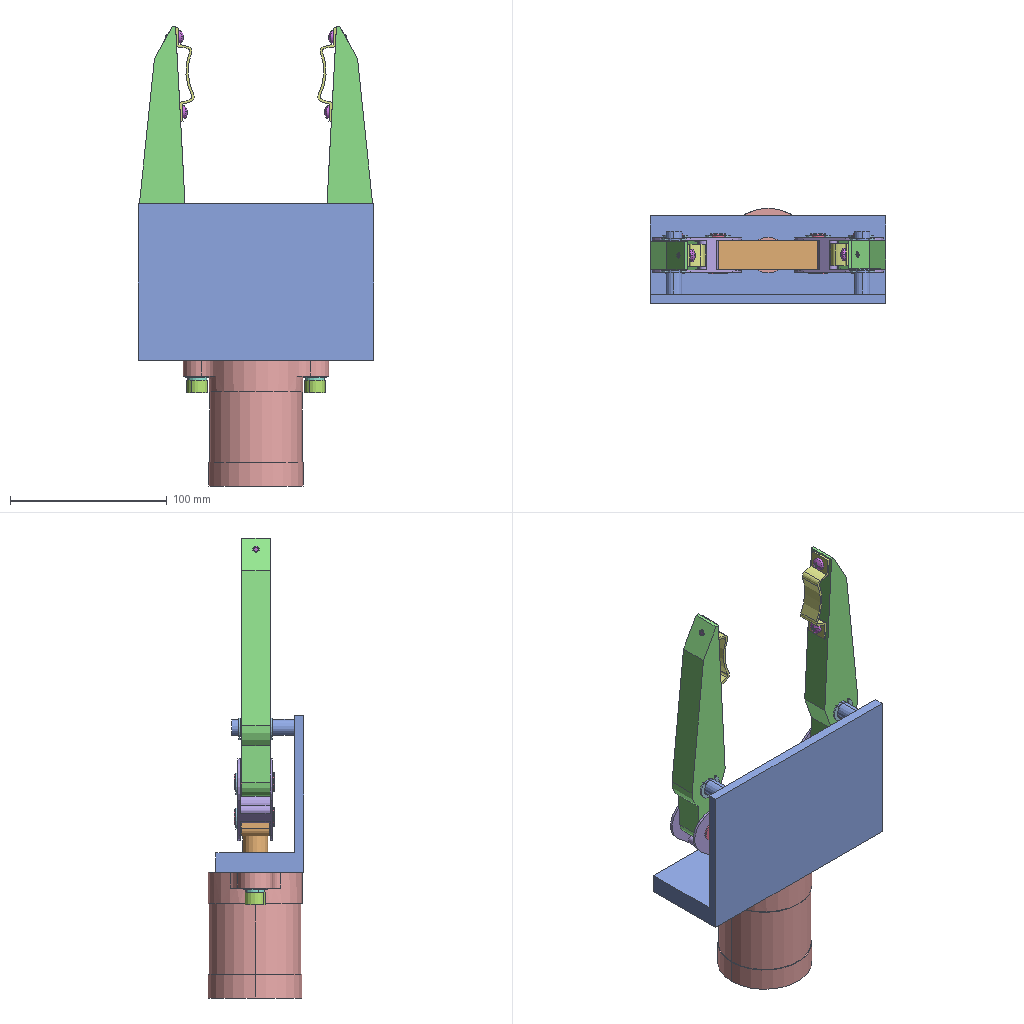Assembly | SolidWorks | 12 different items | 31 placed | box 150 x 61 x 293 mm
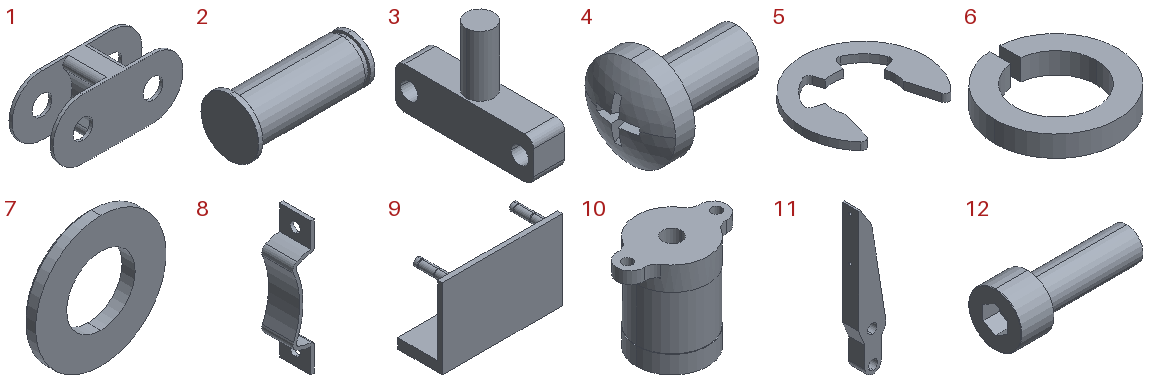Parts list (item | quantity | size | volume | features):
1 | x2 | 65 x 22 x 30 mm | 10120 mm3 | features Extrusion 1, Fillet 1, ICE 1
2 | x4 | 25.5 x 12 x 12 mm | 1834 mm3 | features Chamfer 2, ICE 2, Extrusion 1, Fillet 1
3 | x1 | 18 x 80 x 59 mm | 38383 mm3 | features ICE 2, Extrusion 1, Fillet 1
4 | x4 | 11.081 x 8 x 8 mm | 215 mm3 | features BlendCut 1, LPattern 1, MirrorPattern 1, RevCut 1, Revolution 1
5 | x8 | 16 x 13.638 x 1 mm | 90.427 mm3 | features Extrusion 1
6 | x2 | 12.277 x 12.254 x 2.1 mm | 135.755 mm3 | features Extrusion 1
7 | x2 | 16 x 1.6 x 16 mm | 229.077 mm3 | features Revolution 1
8 | x2 | 9.547 x 14 x 60 mm | 1466 mm3 | features ExtruThin 1, ICE 1
9 | x1 | 150 x 56 x 100 mm | 183819 mm3 | features Cut 3, ICE 2, 3DProfileFeature 1, Extrusion 1, HoleWzd 1
10 | x1 | 92.5 x 60 x 80 mm | 214232 mm3 | features ICE 5, Cut 2, Extrusion 1, Fillet 1
11 | x2 | 30.153 x 18 x 164 mm | 54880 mm3 | features 3DProfileFeature 1, Extrusion 1, HoleWzd 1
12 | x2 | 33 x 13 x 13 mm | 2189 mm3 | features BlendCut 1, Cut 1, Fillet 1, LPattern 1, RevCut 1, Revolution 1
Mates (type | each side: item.copy, entity, surface, feature):
Concentric | 10.1 face cylinder Cut-Extrude1 | 9.1 face cylinder Boss-Extrude1
Coincident | 10.1 face plane Boss-Extrude1 | 9.1 face plane Boss-Extrude1
Concentric | 10.1 face cylinder Cut-Extrude2 | 12.1 face cylinder Base-Revolve
Coincident | 10.1 face plane Cut-Extrude3 | 7.1 face plane Base-Revolve | 2 times
Coincident | 7.1 face plane Base-Revolve | 6.1 face plane Extrude1
Concentric | 7.1 face cylinder Base-Revolve | 6.1 face cylinder Extrude1
Concentric | 10.1 face cylinder Cut-Extrude2 | 6.1 face cylinder Extrude1
Coincident | 12.1 face plane Base-Revolve | 6.1 face plane Extrude1
Concentric | 10.1 face cylinder Cut-Extrude1 | 3.1 face cylinder Boss-Extrude1
Parallel | 9.1 face plane Boss-Extrude2 | 3.1 face plane Boss-Extrude2
Concentric | 3.1 face cylinder Cut-Extrude1 | 1.1 face cylinder Boss-Extrude2
DistanceDim | 1.1 face plane Cut-Extrude1 | 3.1 face plane Boss-Extrude2
DistanceDim | 1.2 face plane Cut-Extrude1 | 3.1 face plane Boss-Extrude2
Concentric | 3.1 face cylinder Cut-Extrude1 | 1.2 face cylinder Boss-Extrude2
Concentric | 1.2 face cylinder Boss-Extrude2 | 11.1 face cylinder Boss-Extrude1
DistanceDim | 11.1 face plane Boss-Extrude1 | 1.2 face plane Cut-Extrude1
Concentric | 10.1 face cylinder Cut-Extrude2 | 9.1 face cylinder M8x1.25 Tapped Hole1
Concentric | 9.1 face cylinder Boss-Extrude3 | 11.1 face cylinder Boss-Extrude1
Coincident | 1.1 face plane Cut-Extrude1 | 11.2 face plane Boss-Extrude1
Concentric | 1.1 face cylinder Boss-Extrude2 | 11.2 face cylinder Boss-Extrude1
Concentric | 9.1 face cylinder Boss-Extrude3 | 11.2 face cylinder Boss-Extrude1
Coincident | 1.1 face plane Boss-Extrude2 | 2.1 face plane Boss-Extrude2
Concentric | 11.2 face cylinder Boss-Extrude1 | 2.1 face cylinder Boss-Extrude1
Concentric | 2.1 face cylinder Cut-Extrude1 | 5.1 face cylinder Extrude1
Coincident | 2.1 face plane Cut-Extrude1 | 5.1 face plane Extrude1
Concentric | 3.1 face cylinder Cut-Extrude1 | 2.2 face cylinder Boss-Extrude1
Coincident | 1.1 face plane Boss-Extrude2 | 2.2 face plane Boss-Extrude2
Concentric | 3.1 face cylinder Cut-Extrude1 | 2.3 face cylinder Boss-Extrude1
Coincident | 1.2 face plane Boss-Extrude2 | 2.3 face plane Boss-Extrude2
Concentric | 11.1 face cylinder Boss-Extrude1 | 2.4 face cylinder Boss-Extrude1
Coincident | 1.2 face plane Boss-Extrude2 | 2.4 face plane Boss-Extrude2
Concentric | 2.4 face cylinder Cut-Extrude1 | 5.2 face cylinder Extrude1
Coincident | 2.4 face plane Cut-Extrude1 | 5.2 face plane Extrude1
Concentric | 2.3 face cylinder Cut-Extrude1 | 5.3 face cylinder Extrude1
Coincident | 2.3 face plane Cut-Extrude1 | 5.3 face plane Extrude1
Concentric | 2.2 face cylinder Cut-Extrude1 | 5.4 face cylinder Extrude1
Coincident | 2.2 face plane Cut-Extrude1 | 5.4 face plane Extrude1
Concentric | 9.1 face cylinder Cut-Extrude1 | 5.5 face cylinder Extrude1
Coincident | 9.1 face plane Cut-Extrude1 | 5.5 face plane Extrude1
Concentric | 9.1 face cylinder Cut-Extrude2 | 5.6 face cylinder Extrude1
Coincident | 9.1 face plane Cut-Extrude2 | 5.6 face plane Extrude1
Concentric | 9.1 face cylinder Cut-Extrude1 | 5.7 face cylinder Extrude1
Coincident | 9.1 face plane Cut-Extrude1 | 5.7 face plane Extrude1
Concentric | 9.1 face cylinder Cut-Extrude2 | 5.8 face cylinder Extrude1
Coincident | 9.1 face plane Cut-Extrude2 | 5.8 face plane Extrude1
Concentric | 11.1 face cylinder M4x0.7 Tapped Hole2 | 4.1 face cylinder Base-Revolve
Coincident | 11.1 face plane Boss-Extrude1 | 8.1 face plane Extrude-Thin3
Concentric | 11.1 face cylinder M4x0.7 Tapped Hole2 | 8.1 face cylinder Cut-Extrude2
Coincident | 8.1 face plane Extrude-Thin3 | 4.1 face plane Base-Revolve
Concentric | 11.1 face cylinder M4x0.7 Tapped Hole2 | 4.2 face cylinder Base-Revolve
Coincident | 8.1 face plane Extrude-Thin3 | 4.2 edge
Coincident | 11.2 face plane Boss-Extrude1 | 8.2 face plane Extrude-Thin3
Concentric | 11.2 face cylinder M4x0.7 Tapped Hole2 | 8.2 face cylinder Cut-Extrude2 | 2 times
Concentric | 11.2 face cylinder M4x0.7 Tapped Hole2 | 4.3 face cylinder Base-Revolve
Coincident | 8.2 face plane Extrude-Thin3 | 4.3 face plane Base-Revolve
Concentric | 11.2 face cylinder M4x0.7 Tapped Hole2 | 4.4 face cylinder Base-Revolve
Coincident | 8.2 face plane Extrude-Thin3 | 4.4 face plane Base-Revolve